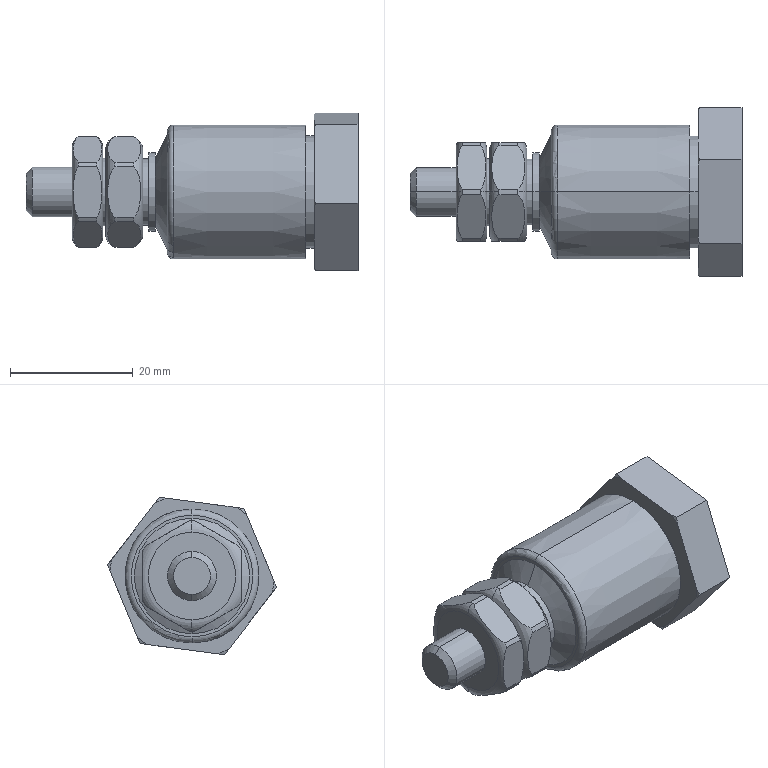Part | SolidWorks | features ICE 2, Revolution 1 | 1 solid | 79 faces | box 54 x 27.472 x 25.615 mm | volume 13856 mm3 | plane 29 | cylinder 26 | torus 16 | cone 8 | commonest cylinder face diameters 18 x14 8 x2 10 x2 10.787 x2 11 x2 12.787 x2